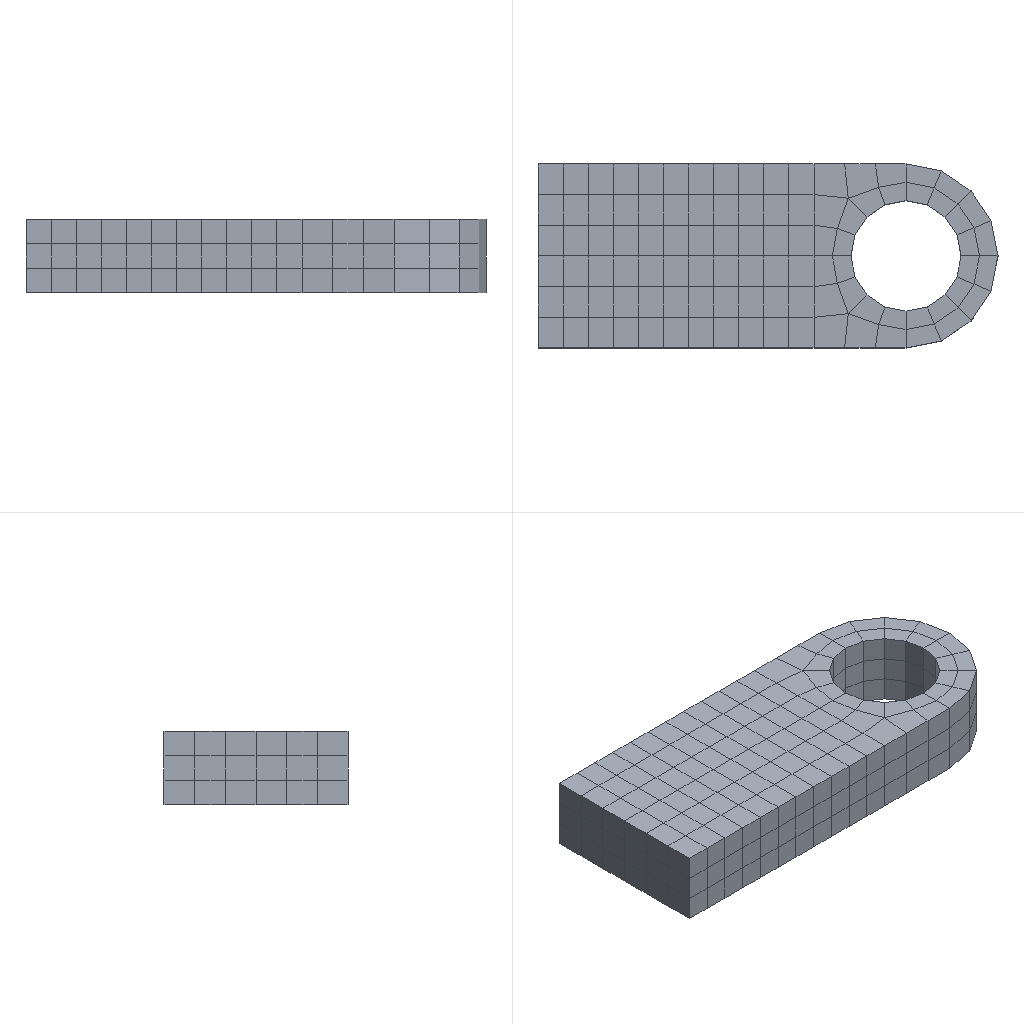Simulation study | abaqus
Set-up summary:
category,name,step,type,value,unit,region
solver,abaqus,,Abaqus/CAE 2024
units,SI m-kg-s (Pa),,inferred,E=2e+11 density=7800
analysis,LugLoad,,dynamic explicit,nlgeom=True; time_period=0.005
mesh,nodes,,,516
mesh,elements,,,300
element_type,C3D8R,,,300
material,Steel,,E,2e+11
material,Steel,,nu,0.3
material,Steel,,density,7800
section,Steel,,solid section,,,_PickedSet2
load,Pressure,LugLoad,pressure,5e+07,,_PickedSurf5
bc,Fix,LugLoad,encastre,[dofs=ENCASTRE],,_PickedSet4
Abaqus input file, long lists of numbers shortened:
*Heading
** Job name: deck Model name: explicit
** Generated by: Abaqus/CAE 2024
*Preprint, echo=NO, model=NO, history=NO, contact=NO
**
** PARTS
**
*Part, name=Lug
*Node
      1, 0.055, 0.015, 0.02
      2, 0.055, 0.015,           0.
** (514 more lines like these left out)
*Element, type=C3D8R
  1,  62, 229, 413, 189,   1,  27, 181,  34
  2, 229, 230, 414, 413,  27,  28, 182, 181
** (298 more lines like these left out)
*Nset, nset=_PickedSet2, internal, generate
   1,  516,    1
*Elset, elset=_PickedSet2, internal, generate
   1,  300,    1
** Section: LugSection
*Solid Section, elset=_PickedSet2, controls=EC-1, material=Steel
1.,
*End Part
**
**
** ASSEMBLY
**
*Assembly, name=Assembly
**
*Instance, name=Lug-1, part=Lug
*End Instance
**
*Nset, nset=_PickedSet4, internal, instance=Lug-1
   5,   6,   7,   8,  17,  18,  35,  36,  37,  38,  39,  40,  41,  42, 115, 116
 127, 128, 131, 132, 185, 186, 187, 188, 353, 354, 355, 356
*Elset, elset=_PickedSet4, internal, instance=Lug-1
  91,  92,  93,  94,  95,  96,  97,  98,  99, 157, 158, 159, 190, 191, 192, 223
 224, 225
*Elset, elset=__PickedSurf5_S3, internal, instance=Lug-1
 280, 281, 295, 296
*Elset, elset=__PickedSurf5_S4, internal, instance=Lug-1, generate
 282,  285,    1
*Elset, elset=__PickedSurf5_S2, internal, instance=Lug-1
 250, 251, 252, 253, 254, 255, 256, 257, 258, 259, 260, 261, 297, 298, 299, 300
*Surface, type=ELEMENT, name=_PickedSurf5, internal
__PickedSurf5_S3, S3
__PickedSurf5_S4, S4
__PickedSurf5_S2, S2
*End Assembly
**
** ELEMENT CONTROLS
**
*Section Controls, name=EC-1, hourglass=ENHANCED
1., 1., 1.
**
** MATERIALS
**
*Material, name=Steel
*Density
7800.,
*Elastic
 2e+11, 0.3
** ----------------------------------------------------------------
**
** STEP: LugLoad
**
*Step, name=LugLoad, nlgeom=YES
*Dynamic, Explicit
, 0.005
*Bulk Viscosity
0.06, 1.2
**
** BOUNDARY CONDITIONS
**
** Name: Fix left end Type: Symmetry/Antisymmetry/Encastre
*Boundary
_PickedSet4, ENCASTRE
**
** LOADS
**
** Name: Pressure load   Type: Pressure
*Dsload
_PickedSurf5, P, 5e+07
**
** OUTPUT REQUESTS
**
*Restart, write, number interval=1, time marks=NO
**
** FIELD OUTPUT: F-Output-1
**
*Output, field, number interval=125
*Node Output
RF, U
*Element Output, directions=YES
NFORC, S
**
** HISTORY OUTPUT: H-Output-1
**
*Output, history, variable=PRESELECT
*End Step
Results summary:
result,odb.job_status,,,JOB_STATUS_COMPLETED_SUCCESSFULLY,"consistent, unstated (Abaqus has no unit system)"
result,steps[0].procedure,LugLoad,,"*DYNAMIC, EXPLICIT","consistent, unstated (Abaqus has no unit system)"
result,steps[0].time_period,LugLoad,,0.005,"consistent, unstated (Abaqus has no unit system)"
result,steps[0].n_frames,LugLoad,,126,"consistent, unstated (Abaqus has no unit system)"
result,steps[0].last_frame.id,LugLoad,,6792,"consistent, unstated (Abaqus has no unit system)"
result,steps[0].last_frame.value,LugLoad,,0.005,"consistent, unstated (Abaqus has no unit system)"
result,steps[0].last_frame.description,LugLoad,,Increment      6792: Step Time =   5.0000E-03,"consistent, unstated (Abaqus has no unit system)"
result,steps[0].completed,LugLoad,,True,"consistent, unstated (Abaqus has no unit system)"
result,steps[0].max_U_magnitude,LugLoad,,0.0006278,"consistent, unstated (Abaqus has no unit system)"
result,steps[0].max_S_mises,LugLoad,,4.3065e+08,"consistent, unstated (Abaqus has no unit system)"
result,steps[0].RF_sum[1],LugLoad,,-1650.39,"consistent, unstated (Abaqus has no unit system)"
result,steps[0].RF_sum[2],LugLoad,,43469.9,"consistent, unstated (Abaqus has no unit system)"
result,steps[0].RF_sum[3],LugLoad,,-32.102,"consistent, unstated (Abaqus has no unit system)"
result,steps[0].diagnostic.n_increments,LugLoad,,126,"consistent, unstated (Abaqus has no unit system)"